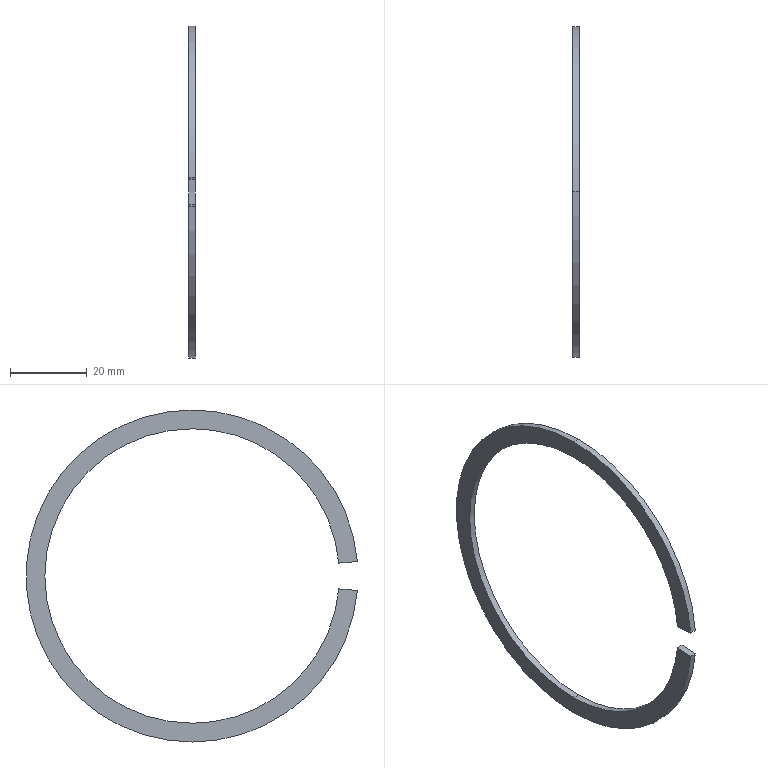Part | STEP file | 0229_Z_B6010ZZNR_2 | 1 solid | 10 faces | box 1.7 x 86.435 x 86.6 mm | volume 2077 mm3 | cylinder 6 | plane 4 | commonest cylinder face diameters 76.81 x3 86.6 x3
STEP:
#1=CARTESIAN_POINT('',(0.,0.,0.));
#2=DIRECTION('',(0.,0.,1.));
#3=DIRECTION('',(1.,0.,0.));
#4=AXIS2_PLACEMENT_3D('',#1,#2,#3);
#5=CARTESIAN_POINT('',(4.98,-38.259,-3.347));
#6=VERTEX_POINT('',#5);
#7=CARTESIAN_POINT('',(3.28,-38.259,-3.347));
#8=VERTEX_POINT('',#7);
#9=CARTESIAN_POINT('',(3.28,-38.259,-3.347));
#10=DIRECTION('',(-1.,0.,0.));
#11=VECTOR('',#10,1.);
#12=LINE('',#9,#11);
#13=CARTESIAN_POINT('',(3.28,0.,0.));
#14=DIRECTION('',(-1.,0.,0.));
#15=DIRECTION('',(0.,0.,1.));
#16=AXIS2_PLACEMENT_3D('',#13,#14,#15);
#17=CYLINDRICAL_SURFACE('',#16,38.405);
#18=CARTESIAN_POINT('',(4.625,0.));
#19=DIRECTION('',(0.,1.));
#20=VECTOR('',#19,1.);
#21=LINE('',#18,#20);
#22=(GEOMETRIC_REPRESENTATION_CONTEXT(2)PARAMETRIC_REPRESENTATION_CONTEXT()REPRESENTATION_CONTEXT('',''));
#23=DEFINITIONAL_REPRESENTATION('',(#21),#22);
#24=PCURVE('',#17,#23);
#25=CARTESIAN_POINT('',(3.28,-43.135,-3.774));
#26=DIRECTION('',(0.,-0.08716,0.9962));
#27=DIRECTION('',(0.,-0.9962,-0.08716));
#28=AXIS2_PLACEMENT_3D('',#25,#26,#27);
#29=PLANE('',#28);
#30=CARTESIAN_POINT('',(-4.895,0.));
#31=DIRECTION('',(0.,-1.));
#32=VECTOR('',#31,1.);
#33=LINE('',#30,#32);
#34=(GEOMETRIC_REPRESENTATION_CONTEXT(2)PARAMETRIC_REPRESENTATION_CONTEXT()REPRESENTATION_CONTEXT('',''));
#35=DEFINITIONAL_REPRESENTATION('',(#33),#34);
#36=PCURVE('',#29,#35);
#37=SURFACE_CURVE('',#12,(#24,#36),.PCURVE_S1.);
#38=EDGE_CURVE('',#6,#8,#37,.T.);
#39=ORIENTED_EDGE('',*,*,#38,.T.);
#40=CARTESIAN_POINT('',(3.28,0.,-38.405));
#41=VERTEX_POINT('',#40);
#42=CARTESIAN_POINT('',(3.28,0.,0.));
#43=DIRECTION('',(1.,0.,0.));
#44=DIRECTION('',(0.,0.,1.));
#45=AXIS2_PLACEMENT_3D('',#42,#43,#44);
#46=CIRCLE('',#45,38.405);
#47=CARTESIAN_POINT('',(6.283,0.));
#48=DIRECTION('',(-1.,0.));
#49=VECTOR('',#48,1.);
#50=LINE('',#47,#49);
#51=(GEOMETRIC_REPRESENTATION_CONTEXT(2)PARAMETRIC_REPRESENTATION_CONTEXT()REPRESENTATION_CONTEXT('',''));
#52=DEFINITIONAL_REPRESENTATION('',(#50),#51);
#53=PCURVE('',#17,#52);
#54=CARTESIAN_POINT('',(3.28,0.,0.));
#55=DIRECTION('',(1.,0.,0.));
#56=DIRECTION('',(0.,0.,-1.));
#57=AXIS2_PLACEMENT_3D('',#54,#55,#56);
#58=PLANE('',#57);
#59=CARTESIAN_POINT('',(0.,0.));
#60=DIRECTION('',(-1.,0.));
#61=AXIS2_PLACEMENT_2D('',#59,#60);
#62=CIRCLE('',#61,38.405);
#63=(GEOMETRIC_REPRESENTATION_CONTEXT(2)PARAMETRIC_REPRESENTATION_CONTEXT()REPRESENTATION_CONTEXT('',''));
#64=DEFINITIONAL_REPRESENTATION('',(#62),#63);
#65=PCURVE('',#58,#64);
#66=SURFACE_CURVE('',#46,(#53,#65),.PCURVE_S1.);
#67=EDGE_CURVE('',#8,#41,#66,.T.);
#68=ORIENTED_EDGE('',*,*,#67,.T.);
#69=CARTESIAN_POINT('',(4.98,0.,-38.405));
#70=VERTEX_POINT('',#69);
#71=CARTESIAN_POINT('',(3.28,0.,-38.405));
#72=DIRECTION('',(-1.,0.,0.));
#73=VECTOR('',#72,1.);
#74=LINE('',#71,#73);
#75=CARTESIAN_POINT('',(3.142,0.));
#76=DIRECTION('',(0.,1.));
#77=VECTOR('',#76,1.);
#78=LINE('',#75,#77);
#79=(GEOMETRIC_REPRESENTATION_CONTEXT(2)PARAMETRIC_REPRESENTATION_CONTEXT()REPRESENTATION_CONTEXT('',''));
#80=DEFINITIONAL_REPRESENTATION('',(#78),#79);
#81=PCURVE('',#17,#80);
#82=CARTESIAN_POINT('',(3.28,0.,0.));
#83=DIRECTION('',(-1.,0.,0.));
#84=DIRECTION('',(0.,0.,1.));
#85=AXIS2_PLACEMENT_3D('',#82,#83,#84);
#86=CYLINDRICAL_SURFACE('',#85,38.405);
#87=CARTESIAN_POINT('',(3.142,0.));
#88=DIRECTION('',(0.,1.));
#89=VECTOR('',#88,1.);
#90=LINE('',#87,#89);
#91=(GEOMETRIC_REPRESENTATION_CONTEXT(2)PARAMETRIC_REPRESENTATION_CONTEXT()REPRESENTATION_CONTEXT('',''));
#92=DEFINITIONAL_REPRESENTATION('',(#90),#91);
#93=PCURVE('',#86,#92);
#94=SURFACE_CURVE('',#74,(#81,#93),.PCURVE_S1.);
#95=EDGE_CURVE('',#70,#41,#94,.T.);
#96=ORIENTED_EDGE('',*,*,#95,.F.);
#97=CARTESIAN_POINT('',(4.98,0.,0.));
#98=DIRECTION('',(-1.,0.,0.));
#99=DIRECTION('',(0.,0.,1.));
#100=AXIS2_PLACEMENT_3D('',#97,#98,#99);
#101=CIRCLE('',#100,38.405);
#102=CARTESIAN_POINT('',(0.,-1.7));
#103=DIRECTION('',(1.,0.));
#104=VECTOR('',#103,1.);
#105=LINE('',#102,#104);
#106=(GEOMETRIC_REPRESENTATION_CONTEXT(2)PARAMETRIC_REPRESENTATION_CONTEXT()REPRESENTATION_CONTEXT('',''));
#107=DEFINITIONAL_REPRESENTATION('',(#105),#106);
#108=PCURVE('',#17,#107);
#109=CARTESIAN_POINT('',(4.98,0.,0.));
#110=DIRECTION('',(1.,0.,0.));
#111=DIRECTION('',(0.,0.,-1.));
#112=AXIS2_PLACEMENT_3D('',#109,#110,#111);
#113=PLANE('',#112);
#114=CARTESIAN_POINT('',(-38.405,0.));
#115=CARTESIAN_POINT('',(-38.405,66.519));
#116=CARTESIAN_POINT('',(19.203,33.26));
#117=CARTESIAN_POINT('',(76.81,0.));
#118=CARTESIAN_POINT('',(19.203,-33.26));
#119=CARTESIAN_POINT('',(-38.405,-66.519));
#120=CARTESIAN_POINT('',(-38.405,0.));
#121=(BOUNDED_CURVE()B_SPLINE_CURVE(2,(#114,#115,#116,#117,#118,#119,#120),.UNSPECIFIED.,.T.,.F.)B_SPLINE_CURVE_WITH_KNOTS((1,2,2,2,2,1),(-2.094,0.,2.094,4.189,6.283,8.378),.UNSPECIFIED.)CURVE()GEOMETRIC_REPRESENTATION_ITEM()RATIONAL_B_SPLINE_CURVE((1.,0.5,1.,0.5,1.,0.5,1.))REPRESENTATION_ITEM(''));
#122=(GEOMETRIC_REPRESENTATION_CONTEXT(2)PARAMETRIC_REPRESENTATION_CONTEXT()REPRESENTATION_CONTEXT('',''));
#123=DEFINITIONAL_REPRESENTATION('',(#121),#122);
#124=PCURVE('',#113,#123);
#125=SURFACE_CURVE('',#101,(#108,#124),.PCURVE_S1.);
#126=EDGE_CURVE('',#70,#6,#125,.T.);
#127=ORIENTED_EDGE('',*,*,#126,.T.);
#128=EDGE_LOOP('',(#39,#68,#96,#127));
#129=FACE_BOUND('',#128,.F.);
#130=ADVANCED_FACE('',(#129),#17,.F.);
#131=CARTESIAN_POINT('',(3.28,0.,38.405));
#132=VERTEX_POINT('',#131);
#133=CARTESIAN_POINT('',(3.28,0.,0.));
#134=DIRECTION('',(1.,0.,0.));
#135=DIRECTION('',(0.,0.,1.));
#136=AXIS2_PLACEMENT_3D('',#133,#134,#135);
#137=CIRCLE('',#136,38.405);
#138=CARTESIAN_POINT('',(6.283,0.));
#139=DIRECTION('',(-1.,0.));
#140=VECTOR('',#139,1.);
#141=LINE('',#138,#140);
#142=(GEOMETRIC_REPRESENTATION_CONTEXT(2)PARAMETRIC_REPRESENTATION_CONTEXT()REPRESENTATION_CONTEXT('',''));
#143=DEFINITIONAL_REPRESENTATION('',(#141),#142);
#144=PCURVE('',#86,#143);
#145=CARTESIAN_POINT('',(0.,0.));
#146=DIRECTION('',(-1.,0.));
#147=AXIS2_PLACEMENT_2D('',#145,#146);
#148=CIRCLE('',#147,38.405);
#149=(GEOMETRIC_REPRESENTATION_CONTEXT(2)PARAMETRIC_REPRESENTATION_CONTEXT()REPRESENTATION_CONTEXT('',''));
#150=DEFINITIONAL_REPRESENTATION('',(#148),#149);
#151=PCURVE('',#58,#150);
#152=SURFACE_CURVE('',#137,(#144,#151),.PCURVE_S1.);
#153=EDGE_CURVE('',#41,#132,#152,.T.);
#154=ORIENTED_EDGE('',*,*,#153,.T.);
#155=CARTESIAN_POINT('',(4.98,0.,38.405));
#156=VERTEX_POINT('',#155);
#157=CARTESIAN_POINT('',(3.28,0.,38.405));
#158=DIRECTION('',(-1.,0.,0.));
#159=VECTOR('',#158,1.);
#160=LINE('',#157,#159);
#161=CARTESIAN_POINT('',(0.,0.));
#162=DIRECTION('',(0.,1.));
#163=VECTOR('',#162,1.);
#164=LINE('',#161,#163);
#165=(GEOMETRIC_REPRESENTATION_CONTEXT(2)PARAMETRIC_REPRESENTATION_CONTEXT()REPRESENTATION_CONTEXT('',''));
#166=DEFINITIONAL_REPRESENTATION('',(#164),#165);
#167=PCURVE('',#86,#166);
#168=CARTESIAN_POINT('',(3.28,0.,0.));
#169=DIRECTION('',(-1.,0.,0.));
#170=DIRECTION('',(0.,0.,1.));
#171=AXIS2_PLACEMENT_3D('',#168,#169,#170);
#172=CYLINDRICAL_SURFACE('',#171,38.405);
#173=CARTESIAN_POINT('',(6.283,0.));
#174=DIRECTION('',(0.,1.));
#175=VECTOR('',#174,1.);
#176=LINE('',#173,#175);
#177=(GEOMETRIC_REPRESENTATION_CONTEXT(2)PARAMETRIC_REPRESENTATION_CONTEXT()REPRESENTATION_CONTEXT('',''));
#178=DEFINITIONAL_REPRESENTATION('',(#176),#177);
#179=PCURVE('',#172,#178);
#180=SURFACE_CURVE('',#160,(#167,#179),.PCURVE_S1.);
#181=EDGE_CURVE('',#156,#132,#180,.T.);
#182=ORIENTED_EDGE('',*,*,#181,.F.);
#183=CARTESIAN_POINT('',(4.98,0.,0.));
#184=DIRECTION('',(-1.,0.,0.));
#185=DIRECTION('',(0.,0.,1.));
#186=AXIS2_PLACEMENT_3D('',#183,#184,#185);
#187=CIRCLE('',#186,38.405);
#188=CARTESIAN_POINT('',(0.,-1.7));
#189=DIRECTION('',(1.,0.));
#190=VECTOR('',#189,1.);
#191=LINE('',#188,#190);
#192=(GEOMETRIC_REPRESENTATION_CONTEXT(2)PARAMETRIC_REPRESENTATION_CONTEXT()REPRESENTATION_CONTEXT('',''));
#193=DEFINITIONAL_REPRESENTATION('',(#191),#192);
#194=PCURVE('',#86,#193);
#195=CARTESIAN_POINT('',(-38.405,0.));
#196=CARTESIAN_POINT('',(-38.405,66.519));
#197=CARTESIAN_POINT('',(19.203,33.26));
#198=CARTESIAN_POINT('',(76.81,0.));
#199=CARTESIAN_POINT('',(19.203,-33.26));
#200=CARTESIAN_POINT('',(-38.405,-66.519));
#201=CARTESIAN_POINT('',(-38.405,0.));
#202=(BOUNDED_CURVE()B_SPLINE_CURVE(2,(#195,#196,#197,#198,#199,#200,#201),.UNSPECIFIED.,.T.,.F.)B_SPLINE_CURVE_WITH_KNOTS((1,2,2,2,2,1),(-2.094,0.,2.094,4.189,6.283,8.378),.UNSPECIFIED.)CURVE()GEOMETRIC_REPRESENTATION_ITEM()RATIONAL_B_SPLINE_CURVE((1.,0.5,1.,0.5,1.,0.5,1.))REPRESENTATION_ITEM(''));
#203=(GEOMETRIC_REPRESENTATION_CONTEXT(2)PARAMETRIC_REPRESENTATION_CONTEXT()REPRESENTATION_CONTEXT('',''));
#204=DEFINITIONAL_REPRESENTATION('',(#202),#203);
#205=PCURVE('',#113,#204);
#206=SURFACE_CURVE('',#187,(#194,#205),.PCURVE_S1.);
#207=EDGE_CURVE('',#156,#70,#206,.T.);
#208=ORIENTED_EDGE('',*,*,#207,.T.);
#209=ORIENTED_EDGE('',*,*,#95,.T.);
#210=EDGE_LOOP('',(#154,#182,#208,#209));
#211=FACE_BOUND('',#210,.F.);
#212=ADVANCED_FACE('',(#211),#86,.F.);
#213=CARTESIAN_POINT('',(4.98,0.,-43.3));
#214=VERTEX_POINT('',#213);
#215=CARTESIAN_POINT('',(4.98,0.,43.3));
#216=VERTEX_POINT('',#215);
#217=CARTESIAN_POINT('',(4.98,0.,0.));
#218=DIRECTION('',(1.,0.,0.));
#219=DIRECTION('',(0.,0.,1.));
#220=AXIS2_PLACEMENT_3D('',#217,#218,#219);
#221=CIRCLE('',#220,43.3);
#222=CARTESIAN_POINT('',(3.28,0.,0.));
#223=DIRECTION('',(-1.,0.,0.));
#224=DIRECTION('',(0.,0.,1.));
#225=AXIS2_PLACEMENT_3D('',#222,#223,#224);
#226=CYLINDRICAL_SURFACE('',#225,43.3);
#227=CARTESIAN_POINT('',(6.283,-1.7));
#228=DIRECTION('',(-1.,0.));
#229=VECTOR('',#228,1.);
#230=LINE('',#227,#229);
#231=(GEOMETRIC_REPRESENTATION_CONTEXT(2)PARAMETRIC_REPRESENTATION_CONTEXT()REPRESENTATION_CONTEXT('',''));
#232=DEFINITIONAL_REPRESENTATION('',(#230),#231);
#233=PCURVE('',#226,#232);
#234=CARTESIAN_POINT('',(0.,0.));
#235=DIRECTION('',(-1.,0.));
#236=AXIS2_PLACEMENT_2D('',#234,#235);
#237=CIRCLE('',#236,43.3);
#238=(GEOMETRIC_REPRESENTATION_CONTEXT(2)PARAMETRIC_REPRESENTATION_CONTEXT()REPRESENTATION_CONTEXT('',''));
#239=DEFINITIONAL_REPRESENTATION('',(#237),#238);
#240=PCURVE('',#113,#239);
#241=SURFACE_CURVE('',#221,(#233,#240),.PCURVE_S1.);
#242=EDGE_CURVE('',#214,#216,#241,.T.);
#243=ORIENTED_EDGE('',*,*,#242,.F.);
#244=CARTESIAN_POINT('',(3.28,0.,-43.3));
#245=VERTEX_POINT('',#244);
#246=CARTESIAN_POINT('',(3.28,0.,-43.3));
#247=DIRECTION('',(-1.,0.,0.));
#248=VECTOR('',#247,1.);
#249=LINE('',#246,#248);
#250=CARTESIAN_POINT('',(3.142,0.));
#251=DIRECTION('',(0.,1.));
#252=VECTOR('',#251,1.);
#253=LINE('',#250,#252);
#254=(GEOMETRIC_REPRESENTATION_CONTEXT(2)PARAMETRIC_REPRESENTATION_CONTEXT()REPRESENTATION_CONTEXT('',''));
#255=DEFINITIONAL_REPRESENTATION('',(#253),#254);
#256=PCURVE('',#226,#255);
#257=CARTESIAN_POINT('',(3.28,0.,0.));
#258=DIRECTION('',(-1.,0.,0.));
#259=DIRECTION('',(0.,0.,1.));
#260=AXIS2_PLACEMENT_3D('',#257,#258,#259);
#261=CYLINDRICAL_SURFACE('',#260,43.3);
#262=CARTESIAN_POINT('',(3.142,0.));
#263=DIRECTION('',(0.,1.));
#264=VECTOR('',#263,1.);
#265=LINE('',#262,#264);
#266=(GEOMETRIC_REPRESENTATION_CONTEXT(2)PARAMETRIC_REPRESENTATION_CONTEXT()REPRESENTATION_CONTEXT('',''));
#267=DEFINITIONAL_REPRESENTATION('',(#265),#266);
#268=PCURVE('',#261,#267);
#269=SURFACE_CURVE('',#249,(#256,#268),.PCURVE_S1.);
#270=EDGE_CURVE('',#214,#245,#269,.T.);
#271=ORIENTED_EDGE('',*,*,#270,.T.);
#272=CARTESIAN_POINT('',(3.28,0.,43.3));
#273=VERTEX_POINT('',#272);
#274=CARTESIAN_POINT('',(3.28,0.,0.));
#275=DIRECTION('',(1.,0.,0.));
#276=DIRECTION('',(0.,0.,1.));
#277=AXIS2_PLACEMENT_3D('',#274,#275,#276);
#278=CIRCLE('',#277,43.3);
#279=CARTESIAN_POINT('',(6.283,0.));
#280=DIRECTION('',(-1.,0.));
#281=VECTOR('',#280,1.);
#282=LINE('',#279,#281);
#283=(GEOMETRIC_REPRESENTATION_CONTEXT(2)PARAMETRIC_REPRESENTATION_CONTEXT()REPRESENTATION_CONTEXT('',''));
#284=DEFINITIONAL_REPRESENTATION('',(#282),#283);
#285=PCURVE('',#226,#284);
#286=CARTESIAN_POINT('',(0.,0.));
#287=DIRECTION('',(-1.,0.));
#288=AXIS2_PLACEMENT_2D('',#286,#287);
#289=CIRCLE('',#288,43.3);
#290=(GEOMETRIC_REPRESENTATION_CONTEXT(2)PARAMETRIC_REPRESENTATION_CONTEXT()REPRESENTATION_CONTEXT('',''));
#291=DEFINITIONAL_REPRESENTATION('',(#289),#290);
#292=PCURVE('',#58,#291);
#293=SURFACE_CURVE('',#278,(#285,#292),.PCURVE_S1.);
#294=EDGE_CURVE('',#245,#273,#293,.T.);
#295=ORIENTED_EDGE('',*,*,#294,.T.);
#296=CARTESIAN_POINT('',(3.28,0.,43.3));
#297=DIRECTION('',(-1.,0.,0.));
#298=VECTOR('',#297,1.);
#299=LINE('',#296,#298);
#300=CARTESIAN_POINT('',(0.,0.));
#301=DIRECTION('',(0.,1.));
#302=VECTOR('',#301,1.);
#303=LINE('',#300,#302);
#304=(GEOMETRIC_REPRESENTATION_CONTEXT(2)PARAMETRIC_REPRESENTATION_CONTEXT()REPRESENTATION_CONTEXT('',''));
#305=DEFINITIONAL_REPRESENTATION('',(#303),#304);
#306=PCURVE('',#226,#305);
#307=CARTESIAN_POINT('',(3.28,0.,0.));
#308=DIRECTION('',(-1.,0.,0.));
#309=DIRECTION('',(0.,0.,1.));
#310=AXIS2_PLACEMENT_3D('',#307,#308,#309);
#311=CYLINDRICAL_SURFACE('',#310,43.3);
#312=CARTESIAN_POINT('',(6.283,0.));
#313=DIRECTION('',(0.,1.));
#314=VECTOR('',#313,1.);
#315=LINE('',#312,#314);
#316=(GEOMETRIC_REPRESENTATION_CONTEXT(2)PARAMETRIC_REPRESENTATION_CONTEXT()REPRESENTATION_CONTEXT('',''));
#317=DEFINITIONAL_REPRESENTATION('',(#315),#316);
#318=PCURVE('',#311,#317);
#319=SURFACE_CURVE('',#299,(#306,#318),.PCURVE_S1.);
#320=EDGE_CURVE('',#216,#273,#319,.T.);
#321=ORIENTED_EDGE('',*,*,#320,.F.);
#322=EDGE_LOOP('',(#243,#271,#295,#321));
#323=FACE_BOUND('',#322,.T.);
#324=ADVANCED_FACE('',(#323),#226,.T.);
#325=CARTESIAN_POINT('',(4.98,-43.135,3.774));
#326=VERTEX_POINT('',#325);
#327=CARTESIAN_POINT('',(4.98,0.,0.));
#328=DIRECTION('',(1.,0.,0.));
#329=DIRECTION('',(0.,0.,1.));
#330=AXIS2_PLACEMENT_3D('',#327,#328,#329);
#331=CIRCLE('',#330,43.3);
#332=CARTESIAN_POINT('',(6.283,-1.7));
#333=DIRECTION('',(-1.,0.));
#334=VECTOR('',#333,1.);
#335=LINE('',#332,#334);
#336=(GEOMETRIC_REPRESENTATION_CONTEXT(2)PARAMETRIC_REPRESENTATION_CONTEXT()REPRESENTATION_CONTEXT('',''));
#337=DEFINITIONAL_REPRESENTATION('',(#335),#336);
#338=PCURVE('',#311,#337);
#339=CARTESIAN_POINT('',(0.,0.));
#340=DIRECTION('',(-1.,0.));
#341=AXIS2_PLACEMENT_2D('',#339,#340);
#342=CIRCLE('',#341,43.3);
#343=(GEOMETRIC_REPRESENTATION_CONTEXT(2)PARAMETRIC_REPRESENTATION_CONTEXT()REPRESENTATION_CONTEXT('',''));
#344=DEFINITIONAL_REPRESENTATION('',(#342),#343);
#345=PCURVE('',#113,#344);
#346=SURFACE_CURVE('',#331,(#338,#345),.PCURVE_S1.);
#347=EDGE_CURVE('',#216,#326,#346,.T.);
#348=ORIENTED_EDGE('',*,*,#347,.F.);
#349=ORIENTED_EDGE('',*,*,#320,.T.);
#350=CARTESIAN_POINT('',(3.28,-43.135,3.774));
#351=VERTEX_POINT('',#350);
#352=CARTESIAN_POINT('',(3.28,0.,0.));
#353=DIRECTION('',(1.,0.,0.));
#354=DIRECTION('',(0.,0.,1.));
#355=AXIS2_PLACEMENT_3D('',#352,#353,#354);
#356=CIRCLE('',#355,43.3);
#357=CARTESIAN_POINT('',(6.283,0.));
#358=DIRECTION('',(-1.,0.));
#359=VECTOR('',#358,1.);
#360=LINE('',#357,#359);
#361=(GEOMETRIC_REPRESENTATION_CONTEXT(2)PARAMETRIC_REPRESENTATION_CONTEXT()REPRESENTATION_CONTEXT('',''));
#362=DEFINITIONAL_REPRESENTATION('',(#360),#361);
#363=PCURVE('',#311,#362);
#364=CARTESIAN_POINT('',(0.,0.));
#365=DIRECTION('',(-1.,0.));
#366=AXIS2_PLACEMENT_2D('',#364,#365);
#367=CIRCLE('',#366,43.3);
#368=(GEOMETRIC_REPRESENTATION_CONTEXT(2)PARAMETRIC_REPRESENTATION_CONTEXT()REPRESENTATION_CONTEXT('',''));
#369=DEFINITIONAL_REPRESENTATION('',(#367),#368);
#370=PCURVE('',#58,#369);
#371=SURFACE_CURVE('',#356,(#363,#370),.PCURVE_S1.);
#372=EDGE_CURVE('',#273,#351,#371,.T.);
#373=ORIENTED_EDGE('',*,*,#372,.T.);
#374=CARTESIAN_POINT('',(3.28,-43.135,3.774));
#375=DIRECTION('',(-1.,0.,0.));
#376=VECTOR('',#375,1.);
#377=LINE('',#374,#376);
#378=CARTESIAN_POINT('',(4.8,0.));
#379=DIRECTION('',(0.,1.));
#380=VECTOR('',#379,1.);
#381=LINE('',#378,#380);
#382=(GEOMETRIC_REPRESENTATION_CONTEXT(2)PARAMETRIC_REPRESENTATION_CONTEXT()REPRESENTATION_CONTEXT('',''));
#383=DEFINITIONAL_REPRESENTATION('',(#381),#382);
#384=PCURVE('',#311,#383);
#385=CARTESIAN_POINT('',(3.28,-38.259,3.347));
#386=DIRECTION('',(0.,-0.08716,-0.9962));
#387=DIRECTION('',(0.,0.9962,-0.08716));
#388=AXIS2_PLACEMENT_3D('',#385,#386,#387);
#389=PLANE('',#388);
#390=CARTESIAN_POINT('',(-4.895,0.));
#391=DIRECTION('',(0.,-1.));
#392=VECTOR('',#391,1.);
#393=LINE('',#390,#392);
#394=(GEOMETRIC_REPRESENTATION_CONTEXT(2)PARAMETRIC_REPRESENTATION_CONTEXT()REPRESENTATION_CONTEXT('',''));
#395=DEFINITIONAL_REPRESENTATION('',(#393),#394);
#396=PCURVE('',#389,#395);
#397=SURFACE_CURVE('',#377,(#384,#396),.PCURVE_S1.);
#398=EDGE_CURVE('',#326,#351,#397,.T.);
#399=ORIENTED_EDGE('',*,*,#398,.F.);
#400=EDGE_LOOP('',(#348,#349,#373,#399));
#401=FACE_BOUND('',#400,.T.);
#402=ADVANCED_FACE('',(#401),#311,.T.);
#403=CARTESIAN_POINT('',(4.98,-38.259,3.347));
#404=VERTEX_POINT('',#403);
#405=CARTESIAN_POINT('',(4.98,0.,0.));
#406=DIRECTION('',(-1.,0.,0.));
#407=DIRECTION('',(0.,0.,1.));
#408=AXIS2_PLACEMENT_3D('',#405,#406,#407);
#409=CIRCLE('',#408,38.405);
#410=CARTESIAN_POINT('',(-38.405,0.));
#411=CARTESIAN_POINT('',(-38.405,66.519));
#412=CARTESIAN_POINT('',(19.203,33.26));
#413=CARTESIAN_POINT('',(76.81,0.));
#414=CARTESIAN_POINT('',(19.203,-33.26));
#415=CARTESIAN_POINT('',(-38.405,-66.519));
#416=CARTESIAN_POINT('',(-38.405,0.));
#417=(BOUNDED_CURVE()B_SPLINE_CURVE(2,(#410,#411,#412,#413,#414,#415,#416),.UNSPECIFIED.,.T.,.F.)B_SPLINE_CURVE_WITH_KNOTS((1,2,2,2,2,1),(-2.094,0.,2.094,4.189,6.283,8.378),.UNSPECIFIED.)CURVE()GEOMETRIC_REPRESENTATION_ITEM()RATIONAL_B_SPLINE_CURVE((1.,0.5,1.,0.5,1.,0.5,1.))REPRESENTATION_ITEM(''));
#418=(GEOMETRIC_REPRESENTATION_CONTEXT(2)PARAMETRIC_REPRESENTATION_CONTEXT()REPRESENTATION_CONTEXT('',''));
#419=DEFINITIONAL_REPRESENTATION('',(#417),#418);
#420=PCURVE('',#113,#419);
#421=CARTESIAN_POINT('',(0.,-1.7));
#422=DIRECTION('',(1.,0.));
#423=VECTOR('',#422,1.);
#424=LINE('',#421,#423);
#425=(GEOMETRIC_REPRESENTATION_CONTEXT(2)PARAMETRIC_REPRESENTATION_CONTEXT()REPRESENTATION_CONTEXT('',''));
#426=DEFINITIONAL_REPRESENTATION('',(#424),#425);
#427=PCURVE('',#172,#426);
#428=SURFACE_CURVE('',#409,(#420,#427),.PCURVE_S1.);
#429=EDGE_CURVE('',#404,#156,#428,.T.);
#430=ORIENTED_EDGE('',*,*,#429,.T.);
#431=ORIENTED_EDGE('',*,*,#207,.T.);
#432=ORIENTED_EDGE('',*,*,#126,.T.);
#433=CARTESIAN_POINT('',(4.98,-43.135,-3.774));
#434=VERTEX_POINT('',#433);
#435=CARTESIAN_POINT('',(4.98,-38.259,-3.347));
#436=DIRECTION('',(0.,-0.9962,-0.08716));
#437=VECTOR('',#436,1.);
#438=LINE('',#435,#437);
#439=CARTESIAN_POINT('',(3.347,-38.259));
#440=DIRECTION('',(0.08716,-0.9962));
#441=VECTOR('',#440,1.);
#442=LINE('',#439,#441);
#443=(GEOMETRIC_REPRESENTATION_CONTEXT(2)PARAMETRIC_REPRESENTATION_CONTEXT()REPRESENTATION_CONTEXT('',''));
#444=DEFINITIONAL_REPRESENTATION('',(#442),#443);
#445=PCURVE('',#113,#444);
#446=CARTESIAN_POINT('',(-4.895,1.7));
#447=DIRECTION('',(1.,0.));
#448=VECTOR('',#447,1.);
#449=LINE('',#446,#448);
#450=(GEOMETRIC_REPRESENTATION_CONTEXT(2)PARAMETRIC_REPRESENTATION_CONTEXT()REPRESENTATION_CONTEXT('',''));
#451=DEFINITIONAL_REPRESENTATION('',(#449),#450);
#452=PCURVE('',#29,#451);
#453=SURFACE_CURVE('',#438,(#445,#452),.PCURVE_S1.);
#454=EDGE_CURVE('',#6,#434,#453,.T.);
#455=ORIENTED_EDGE('',*,*,#454,.T.);
#456=CARTESIAN_POINT('',(4.98,0.,0.));
#457=DIRECTION('',(1.,0.,0.));
#458=DIRECTION('',(0.,0.,1.));
#459=AXIS2_PLACEMENT_3D('',#456,#457,#458);
#460=CIRCLE('',#459,43.3);
#461=CARTESIAN_POINT('',(0.,0.));
#462=DIRECTION('',(-1.,0.));
#463=AXIS2_PLACEMENT_2D('',#461,#462);
#464=CIRCLE('',#463,43.3);
#465=(GEOMETRIC_REPRESENTATION_CONTEXT(2)PARAMETRIC_REPRESENTATION_CONTEXT()REPRESENTATION_CONTEXT('',''));
#466=DEFINITIONAL_REPRESENTATION('',(#464),#465);
#467=PCURVE('',#113,#466);
#468=CARTESIAN_POINT('',(6.283,-1.7));
#469=DIRECTION('',(-1.,0.));
#470=VECTOR('',#469,1.);
#471=LINE('',#468,#470);
#472=(GEOMETRIC_REPRESENTATION_CONTEXT(2)PARAMETRIC_REPRESENTATION_CONTEXT()REPRESENTATION_CONTEXT('',''));
#473=DEFINITIONAL_REPRESENTATION('',(#471),#472);
#474=PCURVE('',#261,#473);
#475=SURFACE_CURVE('',#460,(#467,#474),.PCURVE_S1.);
#476=EDGE_CURVE('',#434,#214,#475,.T.);
#477=ORIENTED_EDGE('',*,*,#476,.T.);
#478=ORIENTED_EDGE('',*,*,#242,.T.);
#479=ORIENTED_EDGE('',*,*,#347,.T.);
#480=CARTESIAN_POINT('',(4.98,-43.135,3.774));
#481=DIRECTION('',(0.,0.9962,-0.08716));
#482=VECTOR('',#481,1.);
#483=LINE('',#480,#482);
#484=CARTESIAN_POINT('',(-3.774,-43.135));
#485=DIRECTION('',(0.08716,0.9962));
#486=VECTOR('',#485,1.);
#487=LINE('',#484,#486);
#488=(GEOMETRIC_REPRESENTATION_CONTEXT(2)PARAMETRIC_REPRESENTATION_CONTEXT()REPRESENTATION_CONTEXT('',''));
#489=DEFINITIONAL_REPRESENTATION('',(#487),#488);
#490=PCURVE('',#113,#489);
#491=CARTESIAN_POINT('',(-4.895,1.7));
#492=DIRECTION('',(1.,0.));
#493=VECTOR('',#492,1.);
#494=LINE('',#491,#493);
#495=(GEOMETRIC_REPRESENTATION_CONTEXT(2)PARAMETRIC_REPRESENTATION_CONTEXT()REPRESENTATION_CONTEXT('',''));
#496=DEFINITIONAL_REPRESENTATION('',(#494),#495);
#497=PCURVE('',#389,#496);
#498=SURFACE_CURVE('',#483,(#490,#497),.PCURVE_S1.);
#499=EDGE_CURVE('',#326,#404,#498,.T.);
#500=ORIENTED_EDGE('',*,*,#499,.T.);
#501=EDGE_LOOP('',(#430,#431,#432,#455,#477,#478,#479,#500));
#502=FACE_BOUND('',#501,.T.);
#503=ADVANCED_FACE('',(#502),#113,.T.);
#504=CARTESIAN_POINT('',(3.28,-38.259,3.347));
#505=VERTEX_POINT('',#504);
#506=CARTESIAN_POINT('',(3.28,0.,0.));
#507=DIRECTION('',(1.,0.,0.));
#508=DIRECTION('',(0.,0.,1.));
#509=AXIS2_PLACEMENT_3D('',#506,#507,#508);
#510=CIRCLE('',#509,38.405);
#511=CARTESIAN_POINT('',(6.283,0.));
#512=DIRECTION('',(-1.,0.));
#513=VECTOR('',#512,1.);
#514=LINE('',#511,#513);
#515=(GEOMETRIC_REPRESENTATION_CONTEXT(2)PARAMETRIC_REPRESENTATION_CONTEXT()REPRESENTATION_CONTEXT('',''));
#516=DEFINITIONAL_REPRESENTATION('',(#514),#515);
#517=PCURVE('',#172,#516);
#518=CARTESIAN_POINT('',(0.,0.));
#519=DIRECTION('',(-1.,0.));
#520=AXIS2_PLACEMENT_2D('',#518,#519);
#521=CIRCLE('',#520,38.405);
#522=(GEOMETRIC_REPRESENTATION_CONTEXT(2)PARAMETRIC_REPRESENTATION_CONTEXT()REPRESENTATION_CONTEXT('',''));
#523=DEFINITIONAL_REPRESENTATION('',(#521),#522);
#524=PCURVE('',#58,#523);
#525=SURFACE_CURVE('',#510,(#517,#524),.PCURVE_S1.);
#526=EDGE_CURVE('',#132,#505,#525,.T.);
#527=ORIENTED_EDGE('',*,*,#526,.T.);
#528=CARTESIAN_POINT('',(3.28,-38.259,3.347));
#529=DIRECTION('',(1.,0.,0.));
#530=VECTOR('',#529,1.);
#531=LINE('',#528,#530);
#532=CARTESIAN_POINT('',(4.8,0.));
#533=DIRECTION('',(0.,-1.));
#534=VECTOR('',#533,1.);
#535=LINE('',#532,#534);
#536=(GEOMETRIC_REPRESENTATION_CONTEXT(2)PARAMETRIC_REPRESENTATION_CONTEXT()REPRESENTATION_CONTEXT('',''));
#537=DEFINITIONAL_REPRESENTATION('',(#535),#536);
#538=PCURVE('',#172,#537);
#539=CARTESIAN_POINT('',(0.,0.));
#540=DIRECTION('',(0.,1.));
#541=VECTOR('',#540,1.);
#542=LINE('',#539,#541);
#543=(GEOMETRIC_REPRESENTATION_CONTEXT(2)PARAMETRIC_REPRESENTATION_CONTEXT()REPRESENTATION_CONTEXT('',''));
#544=DEFINITIONAL_REPRESENTATION('',(#542),#543);
#545=PCURVE('',#389,#544);
#546=SURFACE_CURVE('',#531,(#538,#545),.PCURVE_S1.);
#547=EDGE_CURVE('',#505,#404,#546,.T.);
#548=ORIENTED_EDGE('',*,*,#547,.T.);
#549=ORIENTED_EDGE('',*,*,#429,.T.);
#550=ORIENTED_EDGE('',*,*,#181,.T.);
#551=EDGE_LOOP('',(#527,#548,#549,#550));
#552=FACE_BOUND('',#551,.F.);
#553=ADVANCED_FACE('',(#552),#172,.F.);
#554=CARTESIAN_POINT('',(3.28,-38.259,3.347));
#555=DIRECTION('',(0.,0.9962,-0.08716));
#556=VECTOR('',#555,1.);
#557=LINE('',#554,#556);
#558=CARTESIAN_POINT('',(0.,0.));
#559=DIRECTION('',(1.,0.));
#560=VECTOR('',#559,1.);
#561=LINE('',#558,#560);
#562=(GEOMETRIC_REPRESENTATION_CONTEXT(2)PARAMETRIC_REPRESENTATION_CONTEXT()REPRESENTATION_CONTEXT('',''));
#563=DEFINITIONAL_REPRESENTATION('',(#561),#562);
#564=PCURVE('',#389,#563);
#565=CARTESIAN_POINT('',(-3.347,-38.259));
#566=DIRECTION('',(0.08716,0.9962));
#567=VECTOR('',#566,1.);
#568=LINE('',#565,#567);
#569=(GEOMETRIC_REPRESENTATION_CONTEXT(2)PARAMETRIC_REPRESENTATION_CONTEXT()REPRESENTATION_CONTEXT('',''));
#570=DEFINITIONAL_REPRESENTATION('',(#568),#569);
#571=PCURVE('',#58,#570);
#572=SURFACE_CURVE('',#557,(#564,#571),.PCURVE_S1.);
#573=EDGE_CURVE('',#351,#505,#572,.T.);
#574=ORIENTED_EDGE('',*,*,#573,.T.);
#575=ORIENTED_EDGE('',*,*,#547,.T.);
#576=ORIENTED_EDGE('',*,*,#499,.F.);
#577=ORIENTED_EDGE('',*,*,#398,.T.);
#578=EDGE_LOOP('',(#574,#575,#576,#577));
#579=FACE_BOUND('',#578,.T.);
#580=ADVANCED_FACE('',(#579),#389,.T.);
#581=ORIENTED_EDGE('',*,*,#270,.F.);
#582=ORIENTED_EDGE('',*,*,#476,.F.);
#583=CARTESIAN_POINT('',(3.28,-43.135,-3.774));
#584=VERTEX_POINT('',#583);
#585=CARTESIAN_POINT('',(3.28,-43.135,-3.774));
#586=DIRECTION('',(-1.,0.,0.));
#587=VECTOR('',#586,1.);
#588=LINE('',#585,#587);
#589=CARTESIAN_POINT('',(4.625,0.));
#590=DIRECTION('',(0.,1.));
#591=VECTOR('',#590,1.);
#592=LINE('',#589,#591);
#593=(GEOMETRIC_REPRESENTATION_CONTEXT(2)PARAMETRIC_REPRESENTATION_CONTEXT()REPRESENTATION_CONTEXT('',''));
#594=DEFINITIONAL_REPRESENTATION('',(#592),#593);
#595=PCURVE('',#261,#594);
#596=CARTESIAN_POINT('',(0.,0.));
#597=DIRECTION('',(0.,-1.));
#598=VECTOR('',#597,1.);
#599=LINE('',#596,#598);
#600=(GEOMETRIC_REPRESENTATION_CONTEXT(2)PARAMETRIC_REPRESENTATION_CONTEXT()REPRESENTATION_CONTEXT('',''));
#601=DEFINITIONAL_REPRESENTATION('',(#599),#600);
#602=PCURVE('',#29,#601);
#603=SURFACE_CURVE('',#588,(#595,#602),.PCURVE_S1.);
#604=EDGE_CURVE('',#434,#584,#603,.T.);
#605=ORIENTED_EDGE('',*,*,#604,.T.);
#606=CARTESIAN_POINT('',(3.28,0.,0.));
#607=DIRECTION('',(1.,0.,0.));
#608=DIRECTION('',(0.,0.,1.));
#609=AXIS2_PLACEMENT_3D('',#606,#607,#608);
#610=CIRCLE('',#609,43.3);
#611=CARTESIAN_POINT('',(6.283,0.));
#612=DIRECTION('',(-1.,0.));
#613=VECTOR('',#612,1.);
#614=LINE('',#611,#613);
#615=(GEOMETRIC_REPRESENTATION_CONTEXT(2)PARAMETRIC_REPRESENTATION_CONTEXT()REPRESENTATION_CONTEXT('',''));
#616=DEFINITIONAL_REPRESENTATION('',(#614),#615);
#617=PCURVE('',#261,#616);
#618=CARTESIAN_POINT('',(0.,0.));
#619=DIRECTION('',(-1.,0.));
#620=AXIS2_PLACEMENT_2D('',#618,#619);
#621=CIRCLE('',#620,43.3);
#622=(GEOMETRIC_REPRESENTATION_CONTEXT(2)PARAMETRIC_REPRESENTATION_CONTEXT()REPRESENTATION_CONTEXT('',''));
#623=DEFINITIONAL_REPRESENTATION('',(#621),#622);
#624=PCURVE('',#58,#623);
#625=SURFACE_CURVE('',#610,(#617,#624),.PCURVE_S1.);
#626=EDGE_CURVE('',#584,#245,#625,.T.);
#627=ORIENTED_EDGE('',*,*,#626,.T.);
#628=EDGE_LOOP('',(#581,#582,#605,#627));
#629=FACE_BOUND('',#628,.T.);
#630=ADVANCED_FACE('',(#629),#261,.T.);
#631=CARTESIAN_POINT('',(3.28,-43.135,-3.774));
#632=DIRECTION('',(0.,-0.9962,-0.08716));
#633=VECTOR('',#632,1.);
#634=LINE('',#631,#633);
#635=CARTESIAN_POINT('',(0.,0.));
#636=DIRECTION('',(1.,0.));
#637=VECTOR('',#636,1.);
#638=LINE('',#635,#637);
#639=(GEOMETRIC_REPRESENTATION_CONTEXT(2)PARAMETRIC_REPRESENTATION_CONTEXT()REPRESENTATION_CONTEXT('',''));
#640=DEFINITIONAL_REPRESENTATION('',(#638),#639);
#641=PCURVE('',#29,#640);
#642=CARTESIAN_POINT('',(3.774,-43.135));
#643=DIRECTION('',(0.08716,-0.9962));
#644=VECTOR('',#643,1.);
#645=LINE('',#642,#644);
#646=(GEOMETRIC_REPRESENTATION_CONTEXT(2)PARAMETRIC_REPRESENTATION_CONTEXT()REPRESENTATION_CONTEXT('',''));
#647=DEFINITIONAL_REPRESENTATION('',(#645),#646);
#648=PCURVE('',#58,#647);
#649=SURFACE_CURVE('',#634,(#641,#648),.PCURVE_S1.);
#650=EDGE_CURVE('',#8,#584,#649,.T.);
#651=ORIENTED_EDGE('',*,*,#650,.T.);
#652=ORIENTED_EDGE('',*,*,#604,.F.);
#653=ORIENTED_EDGE('',*,*,#454,.F.);
#654=ORIENTED_EDGE('',*,*,#38,.T.);
#655=EDGE_LOOP('',(#651,#652,#653,#654));
#656=FACE_BOUND('',#655,.T.);
#657=ADVANCED_FACE('',(#656),#29,.T.);
#658=ORIENTED_EDGE('',*,*,#650,.F.);
#659=ORIENTED_EDGE('',*,*,#67,.T.);
#660=ORIENTED_EDGE('',*,*,#153,.T.);
#661=ORIENTED_EDGE('',*,*,#526,.T.);
#662=ORIENTED_EDGE('',*,*,#573,.F.);
#663=ORIENTED_EDGE('',*,*,#372,.F.);
#664=ORIENTED_EDGE('',*,*,#294,.F.);
#665=ORIENTED_EDGE('',*,*,#626,.F.);
#666=EDGE_LOOP('',(#658,#659,#660,#661,#662,#663,#664,#665));
#667=FACE_BOUND('',#666,.T.);
#668=ADVANCED_FACE('',(#667),#58,.F.);
#669=CLOSED_SHELL('',(#130,#212,#324,#402,#503,#553,#580,#630,#657,#668));
#670=MANIFOLD_SOLID_BREP('',#669);
#671=(LENGTH_UNIT()NAMED_UNIT(*)SI_UNIT(.MILLI.,.METRE.));
#672=UNCERTAINTY_MEASURE_WITH_UNIT(LENGTH_MEASURE(0.0000001),#671,'','');
#673=(NAMED_UNIT(*)PLANE_ANGLE_UNIT()SI_UNIT($,.RADIAN.));
#674=(NAMED_UNIT(*)SI_UNIT($,.STERADIAN.)SOLID_ANGLE_UNIT());
#675=(GEOMETRIC_REPRESENTATION_CONTEXT(3)GLOBAL_UNCERTAINTY_ASSIGNED_CONTEXT((#672))GLOBAL_UNIT_ASSIGNED_CONTEXT((#671,#673,#674))REPRESENTATION_CONTEXT('',''));
#676=ADVANCED_BREP_SHAPE_REPRESENTATION('',(#4,#670),#675);